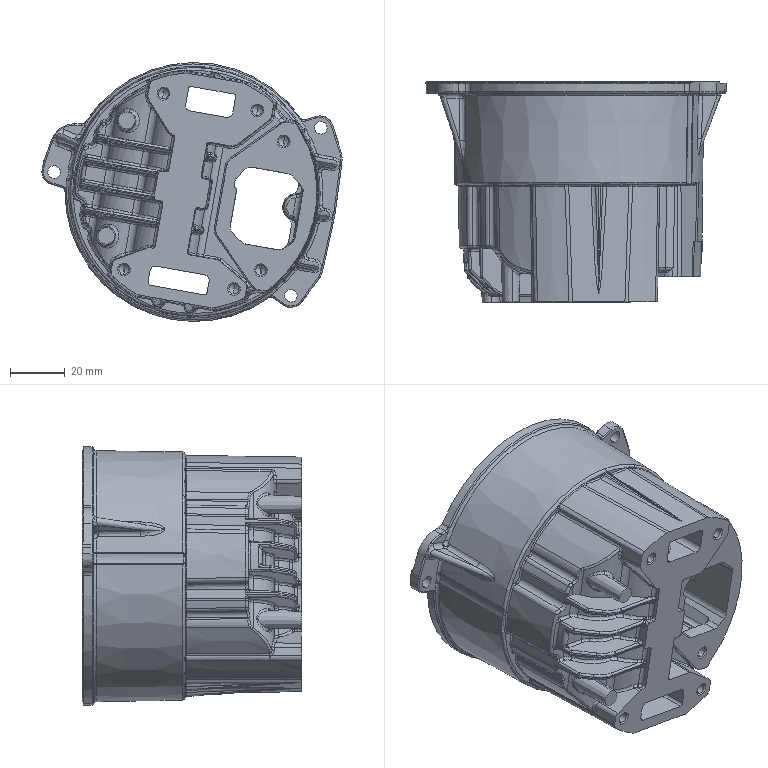Part | SolidWorks | features BaseBody 1 | 1 solid | 2166 faces | box 110.202 x 80.7 x 95 mm | volume 124997 mm3 | plane 932 | spline 565 | cylinder 413 | torus 126 | cone 110 | sphere 20 | commonest cylinder face diameters 2 x86 4 x39 1 x37 3 x30 1.5 x28 6 x22